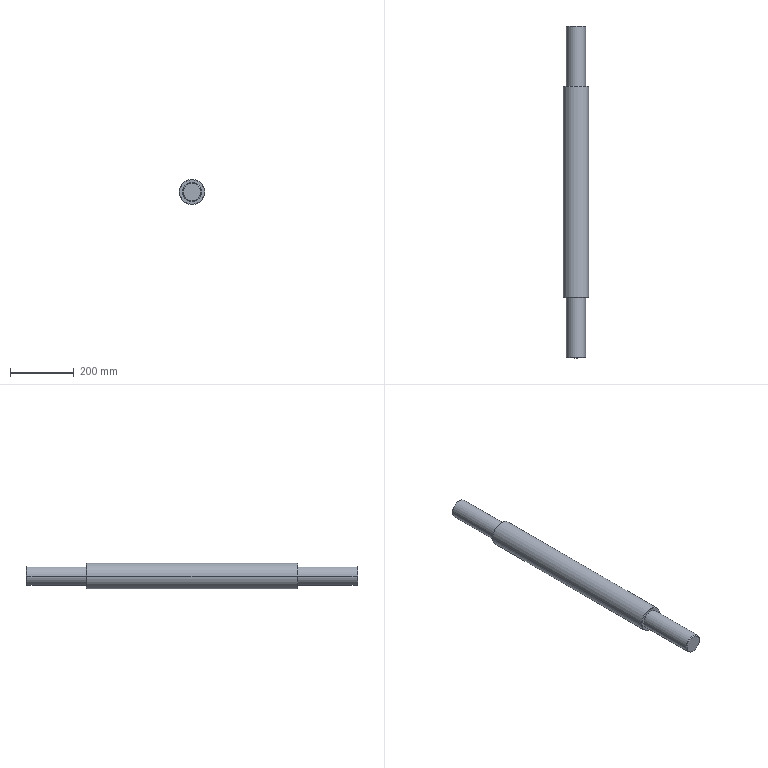Part | SolidWorks | features BaseBody 1 | 1 solid | 18 faces | box 80 x 1045 x 80 mm | volume 4415190 mm3 | cone 8 | cylinder 6 | plane 4 | commonest cylinder face diameters 60 x4 80 x2
STEP:
#1=CARTESIAN_POINT('',(39.,-332.5,0.));
#2=VERTEX_POINT('',#1);
#3=CARTESIAN_POINT('',(-39.,-332.5,0.));
#4=VERTEX_POINT('',#3);
#5=CARTESIAN_POINT('',(0.,-332.5,0.));
#6=DIRECTION('',(0.,-1.,0.));
#7=DIRECTION('',(-1.,0.,0.));
#8=AXIS2_PLACEMENT_3D('',#5,#6,#7);
#9=CIRCLE('',#8,39.);
#10=EDGE_CURVE('',#2,#4,#9,.T.);
#11=ORIENTED_EDGE('',*,*,#10,.F.);
#12=CARTESIAN_POINT('',(40.,-331.5,0.));
#13=VERTEX_POINT('',#12);
#14=CARTESIAN_POINT('',(40.,-331.5,0.));
#15=DIRECTION('',(0.7071,0.7071,0.));
#16=VECTOR('',#15,1000.);
#17=LINE('',#14,#16);
#18=EDGE_CURVE('',#2,#13,#17,.T.);
#19=ORIENTED_EDGE('',*,*,#18,.T.);
#20=CARTESIAN_POINT('',(-40.,-331.5,0.));
#21=VERTEX_POINT('',#20);
#22=CARTESIAN_POINT('',(0.,-331.5,0.));
#23=DIRECTION('',(0.,1.,0.));
#24=DIRECTION('',(-1.,0.,0.));
#25=AXIS2_PLACEMENT_3D('',#22,#23,#24);
#26=CIRCLE('',#25,40.);
#27=EDGE_CURVE('',#21,#13,#26,.T.);
#28=ORIENTED_EDGE('',*,*,#27,.F.);
#29=CARTESIAN_POINT('',(-40.,-331.5,0.));
#30=DIRECTION('',(-0.7071,0.7071,0.));
#31=VECTOR('',#30,1000.);
#32=LINE('',#29,#31);
#33=EDGE_CURVE('',#4,#21,#32,.T.);
#34=ORIENTED_EDGE('',*,*,#33,.F.);
#35=EDGE_LOOP('',(#11,#19,#28,#34));
#36=FACE_OUTER_BOUND('',#35,.T.);
#37=CARTESIAN_POINT('',(0.,-331.5,0.));
#38=DIRECTION('',(0.,1.,0.));
#39=DIRECTION('',(-1.,0.,0.));
#40=AXIS2_PLACEMENT_3D('',#37,#38,#39);
#41=CONICAL_SURFACE('',#40,40.,0.7854);
#42=ADVANCED_FACE('',(#36),#41,.T.);
#43=CARTESIAN_POINT('',(-39.,332.5,0.));
#44=VERTEX_POINT('',#43);
#45=CARTESIAN_POINT('',(39.,332.5,0.));
#46=VERTEX_POINT('',#45);
#47=CARTESIAN_POINT('',(0.,332.5,0.));
#48=DIRECTION('',(0.,1.,0.));
#49=DIRECTION('',(1.,0.,0.));
#50=AXIS2_PLACEMENT_3D('',#47,#48,#49);
#51=CIRCLE('',#50,39.);
#52=EDGE_CURVE('',#44,#46,#51,.T.);
#53=ORIENTED_EDGE('',*,*,#52,.F.);
#54=CARTESIAN_POINT('',(-40.,331.5,0.));
#55=VERTEX_POINT('',#54);
#56=CARTESIAN_POINT('',(-39.,332.5,0.));
#57=DIRECTION('',(-0.7071,-0.7071,0.));
#58=VECTOR('',#57,1000.);
#59=LINE('',#56,#58);
#60=EDGE_CURVE('',#44,#55,#59,.T.);
#61=ORIENTED_EDGE('',*,*,#60,.T.);
#62=CARTESIAN_POINT('',(40.,331.5,0.));
#63=VERTEX_POINT('',#62);
#64=CARTESIAN_POINT('',(0.,331.5,0.));
#65=DIRECTION('',(0.,-1.,0.));
#66=DIRECTION('',(1.,0.,0.));
#67=AXIS2_PLACEMENT_3D('',#64,#65,#66);
#68=CIRCLE('',#67,40.);
#69=EDGE_CURVE('',#63,#55,#68,.T.);
#70=ORIENTED_EDGE('',*,*,#69,.F.);
#71=CARTESIAN_POINT('',(39.,332.5,0.));
#72=DIRECTION('',(0.7071,-0.7071,0.));
#73=VECTOR('',#72,1000.);
#74=LINE('',#71,#73);
#75=EDGE_CURVE('',#46,#63,#74,.T.);
#76=ORIENTED_EDGE('',*,*,#75,.F.);
#77=EDGE_LOOP('',(#53,#61,#70,#76));
#78=FACE_OUTER_BOUND('',#77,.T.);
#79=CARTESIAN_POINT('',(0.,332.5,0.));
#80=DIRECTION('',(0.,-1.,0.));
#81=DIRECTION('',(1.,0.,0.));
#82=AXIS2_PLACEMENT_3D('',#79,#80,#81);
#83=CONICAL_SURFACE('',#82,39.,0.7854);
#84=ADVANCED_FACE('',(#78),#83,.T.);
#85=CARTESIAN_POINT('',(-27.,522.5,0.));
#86=VERTEX_POINT('',#85);
#87=CARTESIAN_POINT('',(27.,522.5,0.));
#88=VERTEX_POINT('',#87);
#89=CARTESIAN_POINT('',(0.,522.5,0.));
#90=DIRECTION('',(0.,1.,0.));
#91=DIRECTION('',(1.,0.,0.));
#92=AXIS2_PLACEMENT_3D('',#89,#90,#91);
#93=CIRCLE('',#92,27.);
#94=EDGE_CURVE('',#86,#88,#93,.T.);
#95=ORIENTED_EDGE('',*,*,#94,.F.);
#96=CARTESIAN_POINT('',(-30.,519.5,0.));
#97=VERTEX_POINT('',#96);
#98=CARTESIAN_POINT('',(-27.,522.5,0.));
#99=DIRECTION('',(-0.7071,-0.7071,0.));
#100=VECTOR('',#99,1000.);
#101=LINE('',#98,#100);
#102=EDGE_CURVE('',#86,#97,#101,.T.);
#103=ORIENTED_EDGE('',*,*,#102,.T.);
#104=CARTESIAN_POINT('',(30.,519.5,0.));
#105=VERTEX_POINT('',#104);
#106=CARTESIAN_POINT('',(0.,519.5,0.));
#107=DIRECTION('',(0.,-1.,0.));
#108=DIRECTION('',(1.,0.,0.));
#109=AXIS2_PLACEMENT_3D('',#106,#107,#108);
#110=CIRCLE('',#109,30.);
#111=EDGE_CURVE('',#105,#97,#110,.T.);
#112=ORIENTED_EDGE('',*,*,#111,.F.);
#113=CARTESIAN_POINT('',(27.,522.5,0.));
#114=DIRECTION('',(0.7071,-0.7071,0.));
#115=VECTOR('',#114,1000.);
#116=LINE('',#113,#115);
#117=EDGE_CURVE('',#88,#105,#116,.T.);
#118=ORIENTED_EDGE('',*,*,#117,.F.);
#119=EDGE_LOOP('',(#95,#103,#112,#118));
#120=FACE_OUTER_BOUND('',#119,.T.);
#121=CARTESIAN_POINT('',(0.,522.5,0.));
#122=DIRECTION('',(0.,-1.,0.));
#123=DIRECTION('',(1.,0.,0.));
#124=AXIS2_PLACEMENT_3D('',#121,#122,#123);
#125=CONICAL_SURFACE('',#124,27.,0.7854);
#126=ADVANCED_FACE('',(#120),#125,.T.);
#127=CARTESIAN_POINT('',(27.,-522.5,0.));
#128=VERTEX_POINT('',#127);
#129=CARTESIAN_POINT('',(-27.,-522.5,0.));
#130=VERTEX_POINT('',#129);
#131=CARTESIAN_POINT('',(0.,-522.5,0.));
#132=DIRECTION('',(0.,-1.,0.));
#133=DIRECTION('',(-1.,0.,0.));
#134=AXIS2_PLACEMENT_3D('',#131,#132,#133);
#135=CIRCLE('',#134,27.);
#136=EDGE_CURVE('',#128,#130,#135,.T.);
#137=ORIENTED_EDGE('',*,*,#136,.F.);
#138=CARTESIAN_POINT('',(30.,-519.5,0.));
#139=VERTEX_POINT('',#138);
#140=CARTESIAN_POINT('',(30.,-519.5,0.));
#141=DIRECTION('',(0.7071,0.7071,0.));
#142=VECTOR('',#141,1000.);
#143=LINE('',#140,#142);
#144=EDGE_CURVE('',#128,#139,#143,.T.);
#145=ORIENTED_EDGE('',*,*,#144,.T.);
#146=CARTESIAN_POINT('',(-30.,-519.5,0.));
#147=VERTEX_POINT('',#146);
#148=CARTESIAN_POINT('',(0.,-519.5,0.));
#149=DIRECTION('',(0.,1.,0.));
#150=DIRECTION('',(-1.,0.,0.));
#151=AXIS2_PLACEMENT_3D('',#148,#149,#150);
#152=CIRCLE('',#151,30.);
#153=EDGE_CURVE('',#147,#139,#152,.T.);
#154=ORIENTED_EDGE('',*,*,#153,.F.);
#155=CARTESIAN_POINT('',(-30.,-519.5,0.));
#156=DIRECTION('',(-0.7071,0.7071,0.));
#157=VECTOR('',#156,1000.);
#158=LINE('',#155,#157);
#159=EDGE_CURVE('',#130,#147,#158,.T.);
#160=ORIENTED_EDGE('',*,*,#159,.F.);
#161=EDGE_LOOP('',(#137,#145,#154,#160));
#162=FACE_OUTER_BOUND('',#161,.T.);
#163=CARTESIAN_POINT('',(0.,-519.5,0.));
#164=DIRECTION('',(0.,1.,0.));
#165=DIRECTION('',(-1.,0.,0.));
#166=AXIS2_PLACEMENT_3D('',#163,#164,#165);
#167=CONICAL_SURFACE('',#166,30.,0.7854);
#168=ADVANCED_FACE('',(#162),#167,.T.);
#169=CARTESIAN_POINT('',(-30.,332.5,0.));
#170=VERTEX_POINT('',#169);
#171=CARTESIAN_POINT('',(30.,332.5,0.));
#172=VERTEX_POINT('',#171);
#173=CARTESIAN_POINT('',(0.,332.5,0.));
#174=DIRECTION('',(0.,1.,0.));
#175=DIRECTION('',(-1.,0.,0.));
#176=AXIS2_PLACEMENT_3D('',#173,#174,#175);
#177=CIRCLE('',#176,30.);
#178=EDGE_CURVE('',#170,#172,#177,.T.);
#179=ORIENTED_EDGE('',*,*,#178,.T.);
#180=CARTESIAN_POINT('',(30.,522.5,0.));
#181=DIRECTION('',(0.,1.,0.));
#182=VECTOR('',#181,1000.);
#183=LINE('',#180,#182);
#184=EDGE_CURVE('',#172,#105,#183,.T.);
#185=ORIENTED_EDGE('',*,*,#184,.T.);
#186=ORIENTED_EDGE('',*,*,#111,.T.);
#187=CARTESIAN_POINT('',(-30.,522.5,0.));
#188=DIRECTION('',(0.,1.,0.));
#189=VECTOR('',#188,1000.);
#190=LINE('',#187,#189);
#191=EDGE_CURVE('',#170,#97,#190,.T.);
#192=ORIENTED_EDGE('',*,*,#191,.F.);
#193=EDGE_LOOP('',(#179,#185,#186,#192));
#194=FACE_OUTER_BOUND('',#193,.T.);
#195=CARTESIAN_POINT('',(0.,522.5,0.));
#196=DIRECTION('',(0.,1.,0.));
#197=DIRECTION('',(-1.,0.,0.));
#198=AXIS2_PLACEMENT_3D('',#195,#196,#197);
#199=CYLINDRICAL_SURFACE('',#198,30.);
#200=ADVANCED_FACE('',(#194),#199,.T.);
#201=ORIENTED_EDGE('',*,*,#27,.T.);
#202=CARTESIAN_POINT('',(40.,522.5,0.));
#203=DIRECTION('',(0.,1.,0.));
#204=VECTOR('',#203,1000.);
#205=LINE('',#202,#204);
#206=EDGE_CURVE('',#13,#63,#205,.T.);
#207=ORIENTED_EDGE('',*,*,#206,.T.);
#208=ORIENTED_EDGE('',*,*,#69,.T.);
#209=CARTESIAN_POINT('',(-40.,522.5,0.));
#210=DIRECTION('',(0.,1.,0.));
#211=VECTOR('',#210,1000.);
#212=LINE('',#209,#211);
#213=EDGE_CURVE('',#21,#55,#212,.T.);
#214=ORIENTED_EDGE('',*,*,#213,.F.);
#215=EDGE_LOOP('',(#201,#207,#208,#214));
#216=FACE_OUTER_BOUND('',#215,.T.);
#217=CARTESIAN_POINT('',(0.,522.5,0.));
#218=DIRECTION('',(0.,1.,0.));
#219=DIRECTION('',(-1.,0.,0.));
#220=AXIS2_PLACEMENT_3D('',#217,#218,#219);
#221=CYLINDRICAL_SURFACE('',#220,40.);
#222=ADVANCED_FACE('',(#216),#221,.T.);
#223=ORIENTED_EDGE('',*,*,#153,.T.);
#224=CARTESIAN_POINT('',(30.,-332.5,0.));
#225=VERTEX_POINT('',#224);
#226=CARTESIAN_POINT('',(30.,522.5,0.));
#227=DIRECTION('',(0.,1.,0.));
#228=VECTOR('',#227,1000.);
#229=LINE('',#226,#228);
#230=EDGE_CURVE('',#139,#225,#229,.T.);
#231=ORIENTED_EDGE('',*,*,#230,.T.);
#232=CARTESIAN_POINT('',(-30.,-332.5,0.));
#233=VERTEX_POINT('',#232);
#234=CARTESIAN_POINT('',(0.,-332.5,0.));
#235=DIRECTION('',(0.,1.,0.));
#236=DIRECTION('',(-1.,0.,0.));
#237=AXIS2_PLACEMENT_3D('',#234,#235,#236);
#238=CIRCLE('',#237,30.);
#239=EDGE_CURVE('',#233,#225,#238,.T.);
#240=ORIENTED_EDGE('',*,*,#239,.F.);
#241=CARTESIAN_POINT('',(-30.,522.5,0.));
#242=DIRECTION('',(0.,1.,0.));
#243=VECTOR('',#242,1000.);
#244=LINE('',#241,#243);
#245=EDGE_CURVE('',#147,#233,#244,.T.);
#246=ORIENTED_EDGE('',*,*,#245,.F.);
#247=EDGE_LOOP('',(#223,#231,#240,#246));
#248=FACE_OUTER_BOUND('',#247,.T.);
#249=CARTESIAN_POINT('',(0.,522.5,0.));
#250=DIRECTION('',(0.,1.,0.));
#251=DIRECTION('',(-1.,0.,0.));
#252=AXIS2_PLACEMENT_3D('',#249,#250,#251);
#253=CYLINDRICAL_SURFACE('',#252,30.);
#254=ADVANCED_FACE('',(#248),#253,.T.);
#255=CARTESIAN_POINT('',(0.,-522.5,0.));
#256=DIRECTION('',(0.,-1.,0.));
#257=DIRECTION('',(-1.,0.,0.));
#258=AXIS2_PLACEMENT_3D('',#255,#256,#257);
#259=CIRCLE('',#258,27.);
#260=EDGE_CURVE('',#130,#128,#259,.T.);
#261=ORIENTED_EDGE('',*,*,#260,.T.);
#262=ORIENTED_EDGE('',*,*,#136,.T.);
#263=EDGE_LOOP('',(#261,#262));
#264=FACE_OUTER_BOUND('',#263,.T.);
#265=CARTESIAN_POINT('',(30.,-522.5,0.));
#266=DIRECTION('',(0.,1.,0.));
#267=DIRECTION('',(-1.,0.,0.));
#268=AXIS2_PLACEMENT_3D('',#265,#266,#267);
#269=PLANE('',#268);
#270=ADVANCED_FACE('',(#264),#269,.F.);
#271=ORIENTED_EDGE('',*,*,#230,.F.);
#272=CARTESIAN_POINT('',(0.,-519.5,0.));
#273=DIRECTION('',(0.,1.,0.));
#274=DIRECTION('',(-1.,0.,0.));
#275=AXIS2_PLACEMENT_3D('',#272,#273,#274);
#276=CIRCLE('',#275,30.);
#277=EDGE_CURVE('',#139,#147,#276,.T.);
#278=ORIENTED_EDGE('',*,*,#277,.T.);
#279=ORIENTED_EDGE('',*,*,#245,.T.);
#280=CARTESIAN_POINT('',(0.,-332.5,0.));
#281=DIRECTION('',(0.,1.,0.));
#282=DIRECTION('',(-1.,0.,0.));
#283=AXIS2_PLACEMENT_3D('',#280,#281,#282);
#284=CIRCLE('',#283,30.);
#285=EDGE_CURVE('',#225,#233,#284,.T.);
#286=ORIENTED_EDGE('',*,*,#285,.F.);
#287=EDGE_LOOP('',(#271,#278,#279,#286));
#288=FACE_OUTER_BOUND('',#287,.T.);
#289=CARTESIAN_POINT('',(0.,522.5,0.));
#290=DIRECTION('',(0.,1.,0.));
#291=DIRECTION('',(-1.,0.,0.));
#292=AXIS2_PLACEMENT_3D('',#289,#290,#291);
#293=CYLINDRICAL_SURFACE('',#292,30.);
#294=ADVANCED_FACE('',(#288),#293,.T.);
#295=CARTESIAN_POINT('',(0.,-332.5,0.));
#296=DIRECTION('',(0.,-1.,0.));
#297=DIRECTION('',(-1.,0.,0.));
#298=AXIS2_PLACEMENT_3D('',#295,#296,#297);
#299=CIRCLE('',#298,39.);
#300=EDGE_CURVE('',#4,#2,#299,.T.);
#301=ORIENTED_EDGE('',*,*,#300,.T.);
#302=ORIENTED_EDGE('',*,*,#10,.T.);
#303=EDGE_LOOP('',(#301,#302));
#304=FACE_OUTER_BOUND('',#303,.T.);
#305=ORIENTED_EDGE('',*,*,#239,.T.);
#306=ORIENTED_EDGE('',*,*,#285,.T.);
#307=EDGE_LOOP('',(#305,#306));
#308=FACE_BOUND('',#307,.T.);
#309=CARTESIAN_POINT('',(40.,-332.5,0.));
#310=DIRECTION('',(0.,1.,0.));
#311=DIRECTION('',(-1.,0.,0.));
#312=AXIS2_PLACEMENT_3D('',#309,#310,#311);
#313=PLANE('',#312);
#314=ADVANCED_FACE('',(#304,#308),#313,.F.);
#315=ORIENTED_EDGE('',*,*,#206,.F.);
#316=CARTESIAN_POINT('',(0.,-331.5,0.));
#317=DIRECTION('',(0.,1.,0.));
#318=DIRECTION('',(-1.,0.,0.));
#319=AXIS2_PLACEMENT_3D('',#316,#317,#318);
#320=CIRCLE('',#319,40.);
#321=EDGE_CURVE('',#13,#21,#320,.T.);
#322=ORIENTED_EDGE('',*,*,#321,.T.);
#323=ORIENTED_EDGE('',*,*,#213,.T.);
#324=CARTESIAN_POINT('',(0.,331.5,0.));
#325=DIRECTION('',(0.,-1.,0.));
#326=DIRECTION('',(1.,0.,0.));
#327=AXIS2_PLACEMENT_3D('',#324,#325,#326);
#328=CIRCLE('',#327,40.);
#329=EDGE_CURVE('',#55,#63,#328,.T.);
#330=ORIENTED_EDGE('',*,*,#329,.T.);
#331=EDGE_LOOP('',(#315,#322,#323,#330));
#332=FACE_OUTER_BOUND('',#331,.T.);
#333=CARTESIAN_POINT('',(0.,522.5,0.));
#334=DIRECTION('',(0.,1.,0.));
#335=DIRECTION('',(-1.,0.,0.));
#336=AXIS2_PLACEMENT_3D('',#333,#334,#335);
#337=CYLINDRICAL_SURFACE('',#336,40.);
#338=ADVANCED_FACE('',(#332),#337,.T.);
#339=CARTESIAN_POINT('',(0.,332.5,0.));
#340=DIRECTION('',(0.,1.,0.));
#341=DIRECTION('',(1.,0.,0.));
#342=AXIS2_PLACEMENT_3D('',#339,#340,#341);
#343=CIRCLE('',#342,39.);
#344=EDGE_CURVE('',#46,#44,#343,.T.);
#345=ORIENTED_EDGE('',*,*,#344,.T.);
#346=ORIENTED_EDGE('',*,*,#52,.T.);
#347=EDGE_LOOP('',(#345,#346));
#348=FACE_OUTER_BOUND('',#347,.T.);
#349=ORIENTED_EDGE('',*,*,#178,.F.);
#350=CARTESIAN_POINT('',(0.,332.5,0.));
#351=DIRECTION('',(0.,1.,0.));
#352=DIRECTION('',(-1.,0.,0.));
#353=AXIS2_PLACEMENT_3D('',#350,#351,#352);
#354=CIRCLE('',#353,30.);
#355=EDGE_CURVE('',#172,#170,#354,.T.);
#356=ORIENTED_EDGE('',*,*,#355,.F.);
#357=EDGE_LOOP('',(#349,#356));
#358=FACE_BOUND('',#357,.T.);
#359=CARTESIAN_POINT('',(30.,332.5,0.));
#360=DIRECTION('',(0.,-1.,0.));
#361=DIRECTION('',(1.,0.,0.));
#362=AXIS2_PLACEMENT_3D('',#359,#360,#361);
#363=PLANE('',#362);
#364=ADVANCED_FACE('',(#348,#358),#363,.F.);
#365=ORIENTED_EDGE('',*,*,#184,.F.);
#366=ORIENTED_EDGE('',*,*,#355,.T.);
#367=ORIENTED_EDGE('',*,*,#191,.T.);
#368=CARTESIAN_POINT('',(0.,519.5,0.));
#369=DIRECTION('',(0.,-1.,0.));
#370=DIRECTION('',(1.,0.,0.));
#371=AXIS2_PLACEMENT_3D('',#368,#369,#370);
#372=CIRCLE('',#371,30.);
#373=EDGE_CURVE('',#97,#105,#372,.T.);
#374=ORIENTED_EDGE('',*,*,#373,.T.);
#375=EDGE_LOOP('',(#365,#366,#367,#374));
#376=FACE_OUTER_BOUND('',#375,.T.);
#377=CARTESIAN_POINT('',(0.,522.5,0.));
#378=DIRECTION('',(0.,1.,0.));
#379=DIRECTION('',(-1.,0.,0.));
#380=AXIS2_PLACEMENT_3D('',#377,#378,#379);
#381=CYLINDRICAL_SURFACE('',#380,30.);
#382=ADVANCED_FACE('',(#376),#381,.T.);
#383=CARTESIAN_POINT('',(0.,522.5,0.));
#384=DIRECTION('',(0.,1.,0.));
#385=DIRECTION('',(1.,0.,0.));
#386=AXIS2_PLACEMENT_3D('',#383,#384,#385);
#387=CIRCLE('',#386,27.);
#388=EDGE_CURVE('',#88,#86,#387,.T.);
#389=ORIENTED_EDGE('',*,*,#388,.T.);
#390=ORIENTED_EDGE('',*,*,#94,.T.);
#391=EDGE_LOOP('',(#389,#390));
#392=FACE_OUTER_BOUND('',#391,.T.);
#393=CARTESIAN_POINT('',(0.,522.5,0.));
#394=DIRECTION('',(0.,-1.,0.));
#395=DIRECTION('',(1.,0.,0.));
#396=AXIS2_PLACEMENT_3D('',#393,#394,#395);
#397=PLANE('',#396);
#398=ADVANCED_FACE('',(#392),#397,.F.);
#399=ORIENTED_EDGE('',*,*,#144,.F.);
#400=ORIENTED_EDGE('',*,*,#260,.F.);
#401=ORIENTED_EDGE('',*,*,#159,.T.);
#402=ORIENTED_EDGE('',*,*,#277,.F.);
#403=EDGE_LOOP('',(#399,#400,#401,#402));
#404=FACE_OUTER_BOUND('',#403,.T.);
#405=CARTESIAN_POINT('',(0.,-519.5,0.));
#406=DIRECTION('',(0.,1.,0.));
#407=DIRECTION('',(-1.,0.,0.));
#408=AXIS2_PLACEMENT_3D('',#405,#406,#407);
#409=CONICAL_SURFACE('',#408,30.,0.7854);
#410=ADVANCED_FACE('',(#404),#409,.T.);
#411=ORIENTED_EDGE('',*,*,#102,.F.);
#412=ORIENTED_EDGE('',*,*,#388,.F.);
#413=ORIENTED_EDGE('',*,*,#117,.T.);
#414=ORIENTED_EDGE('',*,*,#373,.F.);
#415=EDGE_LOOP('',(#411,#412,#413,#414));
#416=FACE_OUTER_BOUND('',#415,.T.);
#417=CARTESIAN_POINT('',(0.,522.5,0.));
#418=DIRECTION('',(0.,-1.,0.));
#419=DIRECTION('',(1.,0.,0.));
#420=AXIS2_PLACEMENT_3D('',#417,#418,#419);
#421=CONICAL_SURFACE('',#420,27.,0.7854);
#422=ADVANCED_FACE('',(#416),#421,.T.);
#423=ORIENTED_EDGE('',*,*,#60,.F.);
#424=ORIENTED_EDGE('',*,*,#344,.F.);
#425=ORIENTED_EDGE('',*,*,#75,.T.);
#426=ORIENTED_EDGE('',*,*,#329,.F.);
#427=EDGE_LOOP('',(#423,#424,#425,#426));
#428=FACE_OUTER_BOUND('',#427,.T.);
#429=CARTESIAN_POINT('',(0.,332.5,0.));
#430=DIRECTION('',(0.,-1.,0.));
#431=DIRECTION('',(1.,0.,0.));
#432=AXIS2_PLACEMENT_3D('',#429,#430,#431);
#433=CONICAL_SURFACE('',#432,39.,0.7854);
#434=ADVANCED_FACE('',(#428),#433,.T.);
#435=ORIENTED_EDGE('',*,*,#18,.F.);
#436=ORIENTED_EDGE('',*,*,#300,.F.);
#437=ORIENTED_EDGE('',*,*,#33,.T.);
#438=ORIENTED_EDGE('',*,*,#321,.F.);
#439=EDGE_LOOP('',(#435,#436,#437,#438));
#440=FACE_OUTER_BOUND('',#439,.T.);
#441=CARTESIAN_POINT('',(0.,-331.5,0.));
#442=DIRECTION('',(0.,1.,0.));
#443=DIRECTION('',(-1.,0.,0.));
#444=AXIS2_PLACEMENT_3D('',#441,#442,#443);
#445=CONICAL_SURFACE('',#444,40.,0.7854);
#446=ADVANCED_FACE('',(#440),#445,.T.);
#447=CLOSED_SHELL('',(#42,#84,#126,#168,#200,#222,#254,#270,#294,#314,#338,#364,#382,#398,#410,#422,#434,#446));
#448=MANIFOLD_SOLID_BREP('',#447);
#449=CARTESIAN_POINT('',(0.,0.,0.));
#450=DIRECTION('',(0.,0.,1.));
#451=DIRECTION('',(1.,0.,0.));
#452=AXIS2_PLACEMENT_3D('',#449,#450,#451);
#453=(LENGTH_UNIT()NAMED_UNIT(*)SI_UNIT(.MILLI.,.METRE.));
#454=UNCERTAINTY_MEASURE_WITH_UNIT(LENGTH_MEASURE(0.00001),#453,'','');
#455=(NAMED_UNIT(*)PLANE_ANGLE_UNIT()SI_UNIT($,.RADIAN.));
#456=(NAMED_UNIT(*)SI_UNIT($,.STERADIAN.)SOLID_ANGLE_UNIT());
#457=(GEOMETRIC_REPRESENTATION_CONTEXT(3)GLOBAL_UNCERTAINTY_ASSIGNED_CONTEXT((#454))GLOBAL_UNIT_ASSIGNED_CONTEXT((#453,#455,#456))REPRESENTATION_CONTEXT('',''));
#458=ADVANCED_BREP_SHAPE_REPRESENTATION('',(#448,#452),#457);